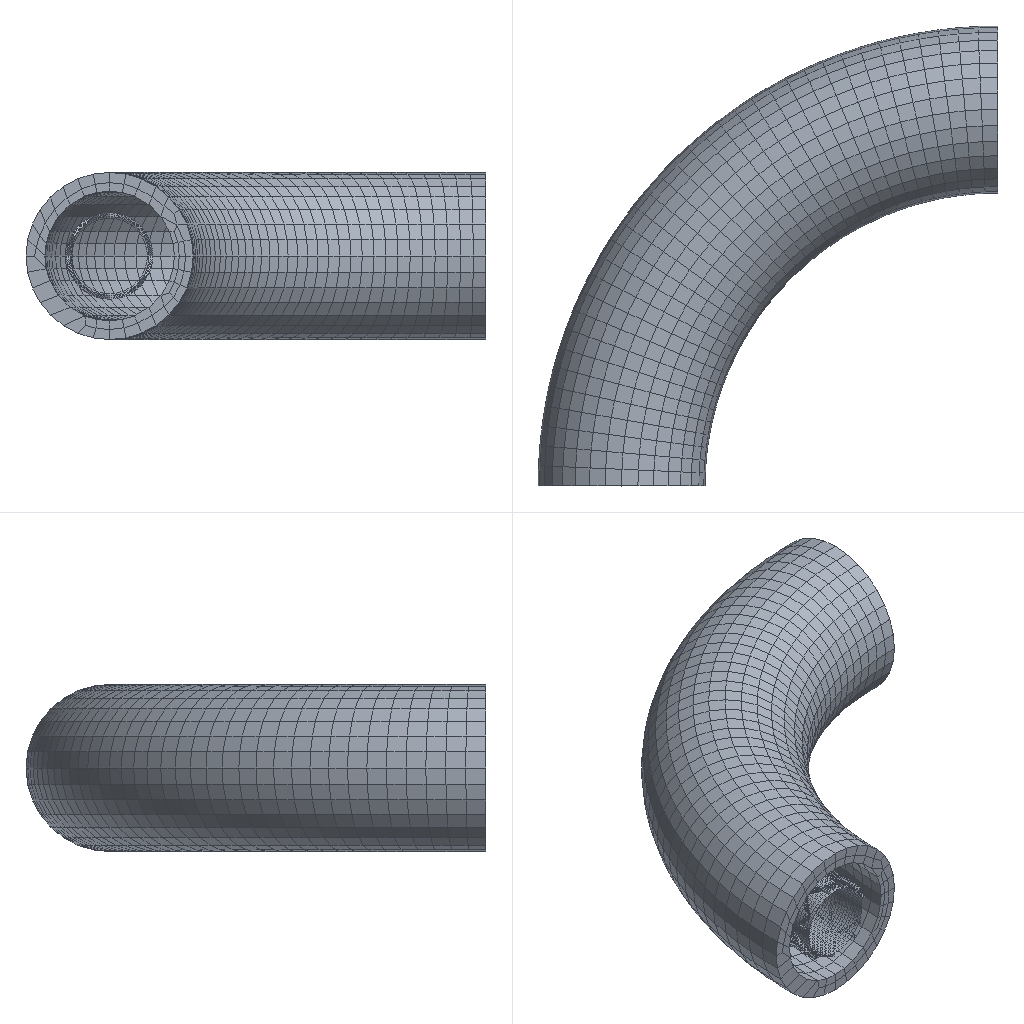Simulation study | abaqus
Set-up summary:
category,name,step,type,value,unit,region
solver,abaqus
solver,version,,,Abaqus/Standard 2020
units,not stated in the deck,,not stated
analysis,deck,,transient,transient
load_step,Step-1,Step-1,transient
load_step,requested,,,1
mesh,nodes,,,9006
mesh,elements,,,15441
element_type,S4R,,shell,1134
element_type,C3D4H,,solid,12039
element_type,C3D8RH,,solid,2268
load,load commands in deck,,count,1
bc,support commands in deck,,count,3
material,SHELL-BALLOON,,in results
material,SS316LN,,in results
material,OGDEN ARTERIAL VESSEL,,in results
check,setup vs results,,match,"per instance, exact: element labels, types and connectivity; labels of the nodes the elements use; coordinates of those nodes at SINGLE_PRECISION in 3 of 3 instance(s)"
Abaqus input file, long lists of numbers shortened:
*Heading
** Job name: Job-1 Model name: Model-1
** Generated by: Abaqus/CAE 2020
*Preprint, echo=NO, model=NO, history=NO, contact=NO
**
** PARTS
**
*Part, name=P05vessel-r10-220518
*Node
      1,  -12.22,           0., -2.5200424e-09
      2,  -12.177,           0.,  0.4331
** (3439 more lines like these left out)
*Element, type=C3D8RH
   1,   68,   66,    1,    2,  161,  159,   94,   95
   2,   34,   66,   68,   33,  127,  159,  161,  126
** (2266 more lines like these left out)
*Nset, nset=Set-1, generate
    1,  3441,     1
*Elset, elset=Set-1, generate
    1,  2268,     1
** Section: Section-2
*Solid Section, elset=Set-1, material="ogden arterial vessel"
,
*End Part
**
*Part, name=Part-1
*Node
      1,  0.995,  0.9, -0.09957
      2,  0.9802,  0.9,  -0.1981
** (1195 more lines like these left out)
*Element, type=S4R
   1,   63,    1,   64,  126
   2,    1,    2,   65,   64
** (1132 more lines like these left out)
*Nset, nset=Set-1, generate
    1,  1197,     1
*Elset, elset=Set-1, generate
    1,  1134,     1
*Nset, nset=Set-3, generate
    1,  1197,     1
*Elset, elset=Set-3, generate
    1,  1134,     1
** Section: Section-1
*Shell Section, elset=Set-1, material=shell-balloon
1., 5
*End Part
**
*Part, name=wrap3layers-R10-220518
*Node
      1, -0.523,  0.55, -0.9058
      2, -0.2032,  0.2828,  -1.026
** (4366 more lines like these left out)
*Element, type=C3D4H
    1, 3584, 3585, 3569, 1457
    2, 3584, 3586,  188, 2546
** (12037 more lines like these left out)
*Nset, nset=Set-1, generate
    1,  4368,     1
*Elset, elset=Set-1, generate
     1,  12039,      1
*Nset, nset=Set-6, generate
    1,  4368,     1
*Elset, elset=Set-6, generate
     1,  12039,      1
** Section: Section-3
*Solid Section, elset=Set-1, material=SS316LN
,
*End Part
**
**
** ASSEMBLY
**
*Assembly, name=Assembly
**
*Instance, name=P05vessel-r10-220518-1, part=P05vessel-r10-220518
   10.11,         -0.9,    -0.284
*End Instance
**
*Instance, name=Part-1-1, part=Part-1
    0.1102,           0.,    -0.284
*End Instance
**
*Instance, name=wrap3layers-R10-220518-1, part=wrap3layers-R10-220518
    0.1102,         -0.9,    -0.284
*End Instance
**
*Nset, nset=Set-1, instance=P05vessel-r10-220518-1, generate
 3349,  3441,     1
*Elset, elset=Set-1, instance=P05vessel-r10-220518-1, generate
 2206,  2268,     1
*Nset, nset=Set-2, instance=Part-1-1, generate
 1135,  1197,     1
*Elset, elset=Set-2, instance=Part-1-1, generate
 1072,  1134,     1
*Nset, nset=Set-3, instance=P05vessel-r10-220518-1, generate
 3349,  3441,     1
*Elset, elset=Set-3, instance=P05vessel-r10-220518-1, generate
 2206,  2268,     1
*Nset, nset=Set-4, instance=Part-1-1, generate
 1135,  1197,     1
*Elset, elset=Set-4, instance=Part-1-1, generate
 1072,  1134,     1
*Nset, nset=Set-5, instance=wrap3layers-R10-220518-1
  135,  136,  137,  138, 1179, 1185
*Elset, elset=Set-5, instance=wrap3layers-R10-220518-1
  2910,  2912, 10089, 10115
*Nset, nset=Set-6, instance=P05vessel-r10-220518-1, generate
  1,  93,   1
*Elset, elset=Set-6, instance=P05vessel-r10-220518-1, generate
  1,  63,   1
*Nset, nset=Set-7, instance=P05vessel-r10-220518-1, generate
  1,  93,   1
*Nset, nset=Set-7, instance=Part-1-1, generate
 1135,  1197,     1
*Elset, elset=Set-7, instance=P05vessel-r10-220518-1, generate
  1,  63,   1
*Elset, elset=Set-7, instance=Part-1-1, generate
 1072,  1134,     1
*Nset, nset=Set-8, instance=P05vessel-r10-220518-1, generate
  1,  93,   1
*Elset, elset=Set-8, instance=P05vessel-r10-220518-1, generate
  1,  63,   1
*Nset, nset=Set-9, instance=Part-1-1, generate
 1135,  1197,     1
*Elset, elset=Set-9, instance=Part-1-1, generate
 1072,  1134,     1
*Elset, elset=_Surf-7_SPOS, internal, instance=Part-1-1, generate
    1,  1134,     1
*Surface, type=ELEMENT, name=Surf-7
_Surf-7_SPOS, SPOS
*Elset, elset=_Surf-8_SPOS, internal, instance=Part-1-1, generate
    1,  1134,     1
*Surface, type=ELEMENT, name=Surf-8
_Surf-8_SPOS, SPOS
*Elset, elset=_Surf-15_SPOS, internal, instance=Part-1-1, generate
    1,  1134,     1
*Surface, type=ELEMENT, name=Surf-15
_Surf-15_SPOS, SPOS
*Elset, elset=_m_Surf-1_SNEG, internal, instance=Part-1-1, generate
    1,  1134,     1
*Surface, type=ELEMENT, name=m_Surf-1
_m_Surf-1_SNEG, SNEG
*Elset, elset=_m_Surf-3_S3, internal, instance=wrap3layers-R10-220518-1
    50,    60,    77,   128,   131,   135,   347,   433,   439,   440,   470,   475,   486,   493,   502,   539
   718,   754,   759,   775,   972,   979,  1011,  1036,  1055,  1083,  1146,  1174,  1237,  1257,  1259,  1315
** (23 more lines like these left out)
*Elset, elset=_m_Surf-3_S1, internal, instance=wrap3layers-R10-220518-1
   284,  5570,  5738,  6653,  7904,  8010,  8072,  8078,  8127,  8131,  8229,  8243,  8525,  8528,  8577,  8584
  8589,  8590,  8594,  8686,  8801,  9018,  9062,  9678,  9724,  9747,  9774,  9791,  9890, 10009, 10609, 10626
** (1 more lines like these left out)
*Elset, elset=_m_Surf-3_S2, internal, instance=wrap3layers-R10-220518-1
  5035,  5699,  5848,  6144,  6166,  6635,  6637,  6676,  6775,  7137,  7143,  7630,  7856,  8003,  8027,  8079
  8312,  8323,  8374,  8539,  8569,  8587,  8682,  8785,  8803,  8981,  8995,  9064,  9143,  9195,  9200,  9247
** (3 more lines like these left out)
*Elset, elset=_m_Surf-3_S4, internal, instance=wrap3layers-R10-220518-1
  5723,  6031,  6055,  6210,  6217,  6370,  6627,  6659,  6682,  7078,  7167,  7181,  7324,  7532,  7582,  7647
  7669,  7969,  8069,  8073,  8088,  8123,  8258,  8298,  8317,  8322,  8330,  8358,  8526,  8601,  8667,  8672
** (5 more lines like these left out)
*Surface, type=ELEMENT, name=m_Surf-3
_m_Surf-3_S3, S3
_m_Surf-3_S1, S1
_m_Surf-3_S2, S2
_m_Surf-3_S4, S4
*Elset, elset=_m_Surf-5_S3, internal, instance=wrap3layers-R10-220518-1
     5,    50,    60,    69,    77,    91,    95,   108,   110,   115,   128,   131,   135,   144,   169,   207
   213,   329,   347,   372,   415,   433,   439,   440,   450,   453,   470,   475,   486,   493,   502,   539
** (49 more lines like these left out)
*Elset, elset=_m_Surf-5_S1, internal, instance=wrap3layers-R10-220518-1
   174,   284,  1690,  3280,  3431,  3438,  3617,  3763,  3976,  3978,  3998,  4007,  4254,  4260,  4271,  4445
  4488,  4647,  4697,  4716,  4773,  4794,  4946,  5128,  5158,  5174,  5238,  5440,  5570,  5595,  5643,  5730
** (4 more lines like these left out)
*Elset, elset=_m_Surf-5_S4, internal, instance=wrap3layers-R10-220518-1
  2001,  3180,  3188,  3224,  3281,  3306,  3631,  3654,  3667,  3755,  3758,  3762,  3766,  3799,  3975,  3987
  3991,  4045,  4231,  4239,  4255,  4264,  4265,  4279,  4282,  4349,  4359,  4362,  4444,  4592,  4638,  4742
** (11 more lines like these left out)
*Elset, elset=_m_Surf-5_S2, internal, instance=wrap3layers-R10-220518-1
  3194,  3651,  3973,  4000,  4038,  4046,  4094,  4138,  4448,  4704,  4728,  4729,  4764,  4784,  4878,  5035
  5093,  5112,  5124,  5143,  5150,  5222,  5229,  5234,  5252,  5334,  5359,  5504,  5556,  5699,  5784,  5785
** (7 more lines like these left out)
*Surface, type=ELEMENT, name=m_Surf-5
_m_Surf-5_S3, S3
_m_Surf-5_S1, S1
_m_Surf-5_S4, S4
_m_Surf-5_S2, S2
*Elset, elset=_m_Surf-9_SNEG, internal, instance=Part-1-1, generate
    1,  1134,     1
*Surface, type=ELEMENT, name=m_Surf-9
_m_Surf-9_SNEG, SNEG
*Elset, elset=_m_Surf-11_SNEG, internal, instance=Part-1-1, generate
    1,  1134,     1
*Surface, type=ELEMENT, name=m_Surf-11
_m_Surf-11_SNEG, SNEG
*Elset, elset=_m_Surf-13_S3, internal, instance=wrap3layers-R10-220518-1
     5,    50,    60,    69,    77,    91,    95,   108,   110,   115,   128,   131,   135,   144,   169,   207
   213,   329,   347,   372,   415,   433,   439,   440,   450,   453,   470,   475,   486,   493,   502,   539
** (49 more lines like these left out)
*Elset, elset=_m_Surf-13_S1, internal, instance=wrap3layers-R10-220518-1
   174,   284,  1690,  3280,  3431,  3438,  3617,  3763,  3976,  3978,  3998,  4007,  4254,  4260,  4271,  4445
  4488,  4647,  4697,  4716,  4773,  4794,  4946,  5128,  5158,  5174,  5238,  5440,  5570,  5595,  5643,  5730
** (4 more lines like these left out)
*Elset, elset=_m_Surf-13_S4, internal, instance=wrap3layers-R10-220518-1
  2001,  3180,  3188,  3224,  3281,  3306,  3631,  3654,  3667,  3755,  3758,  3762,  3766,  3799,  3975,  3987
  3991,  4045,  4231,  4239,  4255,  4264,  4265,  4279,  4282,  4349,  4359,  4362,  4444,  4592,  4638,  4742
** (11 more lines like these left out)
*Elset, elset=_m_Surf-13_S2, internal, instance=wrap3layers-R10-220518-1
  3194,  3651,  3973,  4000,  4038,  4046,  4094,  4138,  4448,  4704,  4728,  4729,  4764,  4784,  4878,  5035
  5093,  5112,  5124,  5143,  5150,  5222,  5229,  5234,  5252,  5334,  5359,  5504,  5556,  5699,  5784,  5785
** (7 more lines like these left out)
*Surface, type=ELEMENT, name=m_Surf-13
_m_Surf-13_S3, S3
_m_Surf-13_S1, S1
_m_Surf-13_S4, S4
_m_Surf-13_S2, S2
*Elset, elset=_m_Surf-16_S4, internal, instance=P05vessel-r10-220518-1
    5,   17,   22,   32,   39,   53,   61,   62,   68,   80,   85,   95,  102,  116,  124,  125
  131,  143,  148,  158,  165,  179,  187,  188,  194,  206,  211,  221,  228,  242,  250,  251
** (16 more lines like these left out)
*Elset, elset=_m_Surf-16_S3, internal, instance=P05vessel-r10-220518-1
    8,   27,   38,   41,   44,   71,   90,  101,  104,  107,  134,  153,  164,  167,  170,  197
  216,  227,  230,  233,  260,  279,  290,  293,  296,  323,  342,  353,  356,  359,  386,  405
** (10 more lines like these left out)
*Elset, elset=_m_Surf-16_S5, internal, instance=P05vessel-r10-220518-1
    9,   28,   37,   43,   45,   46,   47,   58,   60,   72,   91,  100,  106,  108,  109,  110
  121,  123,  135,  154,  163,  169,  171,  172,  173,  184,  186,  198,  217,  226,  232,  234
** (19 more lines like these left out)
*Elset, elset=_m_Surf-16_S6, internal, instance=P05vessel-r10-220518-1
    2,    3,    4,    6,   13,   36,   65,   66,   67,   69,   76,   99,  128,  129,  130,  132
  139,  162,  191,  192,  193,  195,  202,  225,  254,  255,  256,  258,  265,  288,  317,  318
** (12 more lines like these left out)
*Surface, type=ELEMENT, name=m_Surf-16
_m_Surf-16_S4, S4
_m_Surf-16_S3, S3
_m_Surf-16_S6, S6
_m_Surf-16_S5, S5
*Elset, elset=_s_Surf-1_S3, internal, instance=wrap3layers-R10-220518-1
    18,    67,   109,   149,   179,   199,   230,   278,   286,   288,   291,   292,   309,   310,   335,   365
   369,   384,   411,   457,   498,   510,   532,   547,   551,   552,   577,   585,   613,   675,   702,   737
** (54 more lines like these left out)
*Elset, elset=_s_Surf-1_S1, internal, instance=wrap3layers-R10-220518-1
   154,   220,  3101,  3247,  3256,  3276,  3342,  3573,  3671,  3682,  3760,  4061,  4148,  4272,  4392,  4567
  4753,  5162,  5251,  5559,  5874,  5899,  5952,  6123,  6169,  6255,  6491,  6629,  6922,  7002,  7090,  7142
** (2 more lines like these left out)
*Elset, elset=_s_Surf-1_S4, internal, instance=wrap3layers-R10-220518-1
   258,  3048,  3221,  3298,  3301,  3302,  3310,  3320,  3455,  3461,  3499,  3738,  3741,  3747,  3751,  3783
  3802,  4068,  4091,  4243,  4256,  4401,  4545,  4569,  4677,  4909,  4948,  5137,  5191,  5198,  5213,  5444
** (7 more lines like these left out)
*Elset, elset=_s_Surf-1_S2, internal, instance=wrap3layers-R10-220518-1
    58,   308,  2870,  3178,  3229,  3232,  3239,  3442,  3520,  3670,  3773,  3813,  3911,  3957,  4002,  4050
  4228,  4287,  4337,  4384,  4394,  4420,  4588,  4663,  4700,  4774,  4818,  4903,  5087,  5183,  5256,  5304
** (7 more lines like these left out)
*Surface, type=ELEMENT, name=s_Surf-1
_s_Surf-1_S3, S3
_s_Surf-1_S1, S1
_s_Surf-1_S4, S4
_s_Surf-1_S2, S2
*Elset, elset=_s_Surf-3_S6, internal, instance=P05vessel-r10-220518-1
    2,    3,    4,    6,   13,   65,   66,   67,   69,   76,  128,  129,  130,  132,  139,  191
  192,  193,  195,  202,  254,  255,  256,  258,  265,  317,  318,  319,  321,  328,  380,  381
** (10 more lines like these left out)
*Elset, elset=_s_Surf-3_S4, internal, instance=P05vessel-r10-220518-1
    5,   17,   62,   68,   80,  125,  131,  143,  188,  194,  206,  251,  257,  269,  314,  320
  332,  377,  383,  395,  440,  446,  458,  503,  509,  521,  566,  572,  584,  629,  635,  647
** (5 more lines like these left out)
*Elset, elset=_s_Surf-3_S3, internal, instance=P05vessel-r10-220518-1
    8,   41,   44,   71,  104,  107,  134,  167,  170,  197,  230,  233,  260,  293,  296,  323
  356,  359,  386,  419,  422,  449,  482,  485,  512,  545,  548,  575,  608,  611,  638,  671
** (5 more lines like these left out)
*Elset, elset=_s_Surf-3_S5, internal, instance=P05vessel-r10-220518-1
    9,   43,   47,   72,  106,  110,  135,  169,  173,  198,  232,  236,  261,  295,  299,  324
  358,  362,  387,  421,  425,  450,  484,  488,  513,  547,  551,  576,  610,  614,  639,  673
** (5 more lines like these left out)
*Surface, type=ELEMENT, name=s_Surf-3
_s_Surf-3_S6, S6
_s_Surf-3_S4, S4
_s_Surf-3_S3, S3
_s_Surf-3_S5, S5
*Elset, elset=_s_Surf-5_S4, internal, instance=P05vessel-r10-220518-1
    5,   17,   22,   32,   39,   53,   61,   62,   68,   80,   85,   95,  102,  116,  124,  125
  131,  143,  148,  158,  165,  179,  187,  188,  194,  206,  211,  221,  228,  242,  250,  251
** (16 more lines like these left out)
*Elset, elset=_s_Surf-5_S3, internal, instance=P05vessel-r10-220518-1
    8,   27,   38,   41,   44,   71,   90,  101,  104,  107,  134,  153,  164,  167,  170,  197
  216,  227,  230,  233,  260,  279,  290,  293,  296,  323,  342,  353,  356,  359,  386,  405
** (10 more lines like these left out)
*Elset, elset=_s_Surf-5_S5, internal, instance=P05vessel-r10-220518-1
    9,   28,   37,   43,   45,   46,   47,   58,   60,   72,   91,  100,  106,  108,  109,  110
  121,  123,  135,  154,  163,  169,  171,  172,  173,  184,  186,  198,  217,  226,  232,  234
** (19 more lines like these left out)
*Elset, elset=_s_Surf-5_S6, internal, instance=P05vessel-r10-220518-1
    2,    3,    4,    6,   13,   36,   65,   66,   67,   69,   76,   99,  128,  129,  130,  132
  139,  162,  191,  192,  193,  195,  202,  225,  254,  255,  256,  258,  265,  288,  317,  318
** (12 more lines like these left out)
*Surface, type=ELEMENT, name=s_Surf-5
_s_Surf-5_S4, S4
_s_Surf-5_S3, S3
_s_Surf-5_S6, S6
_s_Surf-5_S5, S5
*Elset, elset=_s_Surf-9_S3, internal, instance=wrap3layers-R10-220518-1
    18,    67,   109,   149,   179,   199,   230,   278,   286,   288,   291,   292,   309,   310,   335,   365
   369,   384,   411,   457,   498,   510,   532,   547,   551,   552,   577,   585,   613,   675,   702,   737
** (54 more lines like these left out)
*Elset, elset=_s_Surf-9_S1, internal, instance=wrap3layers-R10-220518-1
   154,   220,  3101,  3247,  3256,  3276,  3342,  3573,  3671,  3682,  3760,  4061,  4148,  4272,  4392,  4567
  4753,  5162,  5251,  5559,  5874,  5899,  5952,  6123,  6169,  6255,  6491,  6629,  6922,  7002,  7090,  7142
** (2 more lines like these left out)
*Elset, elset=_s_Surf-9_S4, internal, instance=wrap3layers-R10-220518-1
   258,  3048,  3221,  3298,  3301,  3302,  3310,  3320,  3455,  3461,  3499,  3738,  3741,  3747,  3751,  3783
  3802,  4068,  4091,  4243,  4256,  4401,  4545,  4569,  4677,  4909,  4948,  5137,  5191,  5198,  5213,  5444
** (7 more lines like these left out)
*Elset, elset=_s_Surf-9_S2, internal, instance=wrap3layers-R10-220518-1
    58,   308,  2870,  3178,  3229,  3232,  3239,  3442,  3520,  3670,  3773,  3813,  3911,  3957,  4002,  4050
  4228,  4287,  4337,  4384,  4394,  4420,  4588,  4663,  4700,  4774,  4818,  4903,  5087,  5183,  5256,  5304
** (7 more lines like these left out)
*Surface, type=ELEMENT, name=s_Surf-9
_s_Surf-9_S3, S3
_s_Surf-9_S1, S1
_s_Surf-9_S4, S4
_s_Surf-9_S2, S2
*Elset, elset=_s_Surf-11_S3, internal, instance=wrap3layers-R10-220518-1
    18,    67,   109,   149,   179,   199,   230,   278,   286,   288,   291,   292,   309,   310,   335,   365
   369,   384,   411,   457,   498,   510,   532,   547,   551,   552,   577,   585,   613,   675,   702,   737
** (54 more lines like these left out)
*Elset, elset=_s_Surf-11_S1, internal, instance=wrap3layers-R10-220518-1
   154,   220,  3101,  3247,  3256,  3276,  3342,  3573,  3671,  3682,  3760,  4061,  4148,  4272,  4392,  4567
  4753,  5162,  5251,  5559,  5874,  5899,  5952,  6123,  6169,  6255,  6491,  6629,  6922,  7002,  7090,  7142
** (2 more lines like these left out)
*Elset, elset=_s_Surf-11_S4, internal, instance=wrap3layers-R10-220518-1
   258,  3048,  3221,  3298,  3301,  3302,  3310,  3320,  3455,  3461,  3499,  3738,  3741,  3747,  3751,  3783
  3802,  4068,  4091,  4243,  4256,  4401,  4545,  4569,  4677,  4909,  4948,  5137,  5191,  5198,  5213,  5444
** (7 more lines like these left out)
*Elset, elset=_s_Surf-11_S2, internal, instance=wrap3layers-R10-220518-1
    58,   308,  2870,  3178,  3229,  3232,  3239,  3442,  3520,  3670,  3773,  3813,  3911,  3957,  4002,  4050
  4228,  4287,  4337,  4384,  4394,  4420,  4588,  4663,  4700,  4774,  4818,  4903,  5087,  5183,  5256,  5304
** (7 more lines like these left out)
*Surface, type=ELEMENT, name=s_Surf-11
_s_Surf-11_S3, S3
_s_Surf-11_S1, S1
_s_Surf-11_S4, S4
_s_Surf-11_S2, S2
*Elset, elset=_s_Surf-13_S4, internal, instance=P05vessel-r10-220518-1
    5,   17,   22,   32,   39,   53,   61,   62,   68,   80,   85,   95,  102,  116,  124,  125
  131,  143,  148,  158,  165,  179,  187,  188,  194,  206,  211,  221,  228,  242,  250,  251
** (16 more lines like these left out)
*Elset, elset=_s_Surf-13_S3, internal, instance=P05vessel-r10-220518-1
    8,   27,   38,   41,   44,   71,   90,  101,  104,  107,  134,  153,  164,  167,  170,  197
  216,  227,  230,  233,  260,  279,  290,  293,  296,  323,  342,  353,  356,  359,  386,  405
** (10 more lines like these left out)
*Elset, elset=_s_Surf-13_S5, internal, instance=P05vessel-r10-220518-1
    9,   28,   37,   43,   45,   46,   47,   58,   60,   72,   91,  100,  106,  108,  109,  110
  121,  123,  135,  154,  163,  169,  171,  172,  173,  184,  186,  198,  217,  226,  232,  234
** (19 more lines like these left out)
*Elset, elset=_s_Surf-13_S6, internal, instance=P05vessel-r10-220518-1
    2,    3,    4,    6,   13,   36,   65,   66,   67,   69,   76,   99,  128,  129,  130,  132
  139,  162,  191,  192,  193,  195,  202,  225,  254,  255,  256,  258,  265,  288,  317,  318
** (12 more lines like these left out)
*Surface, type=ELEMENT, name=s_Surf-13
_s_Surf-13_S4, S4
_s_Surf-13_S3, S3
_s_Surf-13_S6, S6
_s_Surf-13_S5, S5
*Elset, elset=_s_Surf-16_S2, internal, instance=wrap3layers-R10-220518-1
    58,   111,   259,   284,   298,   308,   309,   555,   620,   632,   722,   760,   801,   959,  1072,  1466
  1657,  1672,  1786,  1911,  2354,  2461,  2612,  2642,  2870,  2948,  2994,  3060,  3136,  3178,  3184,  3194
** (49 more lines like these left out)
*Elset, elset=_s_Surf-16_S3, internal, instance=wrap3layers-R10-220518-1
     3,     5,    17,    18,    23,    24,    32,    35,    37,    40,    46,    48,    50,    60,    66,    67
    69,    74,    77,    80,    87,    91,    92,    95,    98,   102,   108,   109,   110,   114,   115,   121
** (311 more lines like these left out)
*Elset, elset=_s_Surf-16_S4, internal, instance=wrap3layers-R10-220518-1
   174,   258,   827,  1414,  1670,  1681,  1690,  1985,  2001,  2312,  3048,  3091,  3166,  3180,  3188,  3189
  3191,  3192,  3194,  3221,  3224,  3225,  3237,  3238,  3280,  3281,  3282,  3298,  3300,  3301,  3302,  3304
** (49 more lines like these left out)
*Elset, elset=_s_Surf-16_S1, internal, instance=wrap3layers-R10-220518-1
    63,   154,   174,   220,   258,   284,   385,   690,  1506,  1690,  1918,  1987,  2317,  3088,  3101,  3178
  3180,  3181,  3188,  3227,  3243,  3247,  3252,  3255,  3256,  3259,  3261,  3262,  3263,  3275,  3276,  3280
** (35 more lines like these left out)
*Surface, type=ELEMENT, name=s_Surf-16
_s_Surf-16_S2, S2
_s_Surf-16_S3, S3
_s_Surf-16_S4, S4
_s_Surf-16_S1, S1
*Elset, elset=_s_Surf-18_SNEG, internal, instance=Part-1-1, generate
    1,  1134,     1
*Surface, type=ELEMENT, name=s_Surf-18
_s_Surf-18_SNEG, SNEG
*End Assembly
*Amplitude, name=Amp-1
             0.,              0.,            0.08,              1.,             0.1,              0.
**
** MATERIALS
**
*Material, name=SS316LN
*Density
 7.99e-09,
*Elastic
196000., 0.3
*Plastic
205.,    0.
515., 0.599
*Material, name="ogden arterial vessel"
*Density
 1.07e-09,
*Hyperelastic, n=3, ogden
 -4.73,    -0.39,      1.7,     4.41,     3.09,    -3.25, 3.63e-06,       0.
       0.,
*Material, name=shell-balloon
*Density
 1.07e-09,
*Elastic
2580., 0.46
**
** INTERACTION PROPERTIES
**
*Surface Interaction, name=IntProp-1
1.,
*Friction, slip tolerance=0.005
 0.15,
*Surface Behavior, pressure-overclosure=HARD
**
** INTERACTIONS
**
** Interaction: Int-5
*Contact Pair, interaction=IntProp-1, type=SURFACE TO SURFACE
s_Surf-16, m_Surf-16
** Interaction: Int-6
*Contact Pair, interaction=IntProp-1, type=SURFACE TO SURFACE
s_Surf-18, s_Surf-16
** ----------------------------------------------------------------
**
** STEP: Step-1
**
*Step, name=Step-1, nlgeom=YES, inc=10000
*Dynamic
0.001,0.1,1e-06
**
** BOUNDARY CONDITIONS
**
** Name: BC-1 Type: 对称/反对称/完全固定
*Boundary
Set-3, ENCASTRE
** Name: BC-3 Type: 对称/反对称/完全固定
*Boundary
Set-8, YSYMM
** Name: BC-4 Type: 对称/反对称/完全固定
*Boundary
Set-9, ENCASTRE
**
** LOADS
**
** Name: Load-1   Type: Pressure
*Dsload, amplitude=Amp-1
Surf-15, P, 20.
**
** OUTPUT REQUESTS
**
*Restart, write, number interval=1, time marks=NO
**
** FIELD OUTPUT: F-Output-1
**
*Output, field, frequency=2
*Node Output
A, CF, RF, U, V
*Element Output, directions=YES
E, LE, MISES, MISESMAX, PE, PEEQ, PEMAG, S, SSAVG
*Contact Output
CDISP, CSTRESS
**
** HISTORY OUTPUT: H-Output-1
**
*Output, history, variable=PRESELECT, number interval=200, time marks=NO
*End Step
Results summary:
result,step,,partial,increments=0 time=0.0/0.1
result,analysis,,,transient
result,last_loadstep,,,1
result,primary field,,,"U, UR"
result,reaction total,,FX,0.0,model units
result,reaction total,,FY,0.0,model units
result,reaction total,,FZ,0.0,model units